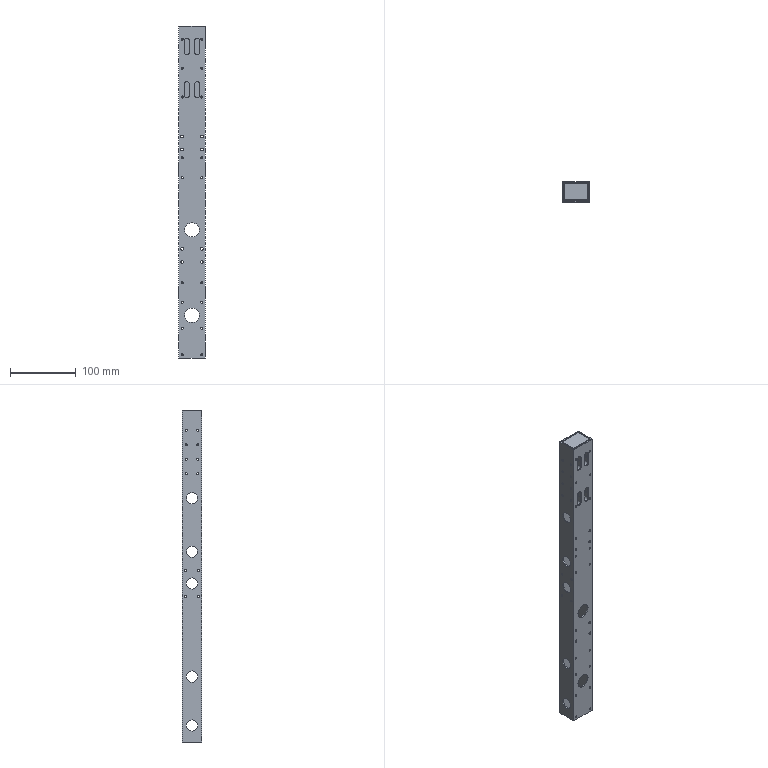Part | SolidWorks | features ICE 9, Chamfer 1, Extrusion 1, Fillet 1 | 2 solids | 317 faces | box 40 x 30 x 505 mm | volume 171270 mm3 | cylinder 263 | plane 54 | commonest cylinder face diameters 3.2 x172 4.2 x32 17 x20 8 x16 8.4 x12 22 x11